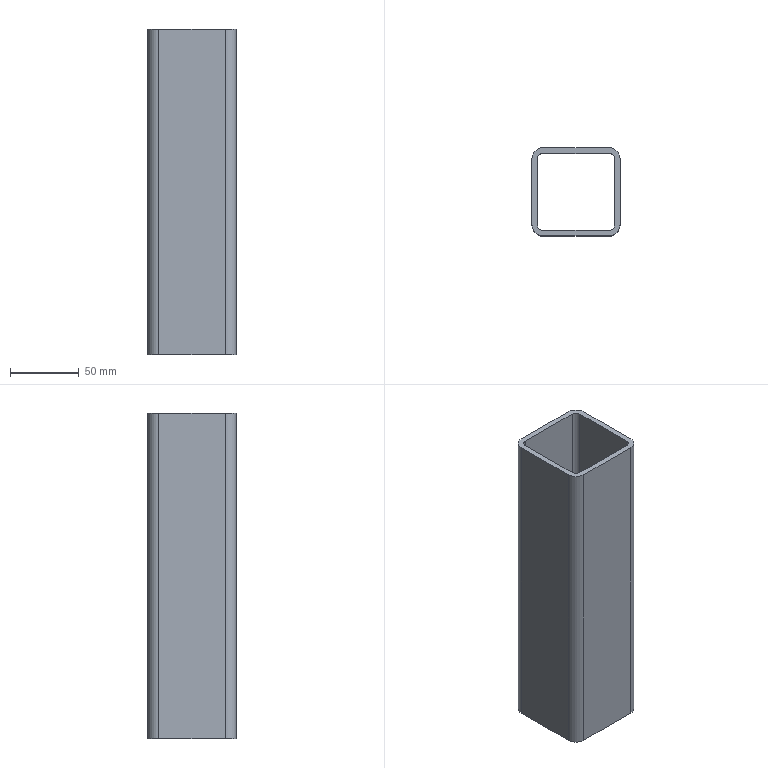Part | SolidWorks | features Extrusion 1 | 1 solid | 18 faces | box 64 x 64 x 236 mm | volume 216836 mm3 | plane 10 | cylinder 8 | commonest cylinder face diameters 8 x4 16 x4
STEP:
#1=CARTESIAN_POINT('',(-24.,32.,118.));
#2=VERTEX_POINT('',#1);
#3=CARTESIAN_POINT('',(-32.,24.,118.));
#4=VERTEX_POINT('',#3);
#5=CARTESIAN_POINT('',(-24.,24.,118.));
#6=DIRECTION('',(0.,0.,1.));
#7=DIRECTION('',(1.,0.,0.));
#8=AXIS2_PLACEMENT_3D('',#5,#6,#7);
#9=CIRCLE('',#8,8.);
#10=EDGE_CURVE('',#2,#4,#9,.T.);
#11=ORIENTED_EDGE('',*,*,#10,.T.);
#12=CARTESIAN_POINT('',(-32.,-24.,118.));
#13=VERTEX_POINT('',#12);
#14=CARTESIAN_POINT('',(-32.,24.,118.));
#15=DIRECTION('',(0.,-1.,0.));
#16=VECTOR('',#15,1000.);
#17=LINE('',#14,#16);
#18=EDGE_CURVE('',#4,#13,#17,.T.);
#19=ORIENTED_EDGE('',*,*,#18,.T.);
#20=CARTESIAN_POINT('',(-24.,-32.,118.));
#21=VERTEX_POINT('',#20);
#22=CARTESIAN_POINT('',(-24.,-24.,118.));
#23=DIRECTION('',(0.,0.,1.));
#24=DIRECTION('',(-1.,0.,0.));
#25=AXIS2_PLACEMENT_3D('',#22,#23,#24);
#26=CIRCLE('',#25,8.);
#27=EDGE_CURVE('',#13,#21,#26,.T.);
#28=ORIENTED_EDGE('',*,*,#27,.T.);
#29=CARTESIAN_POINT('',(24.,-32.,118.));
#30=VERTEX_POINT('',#29);
#31=CARTESIAN_POINT('',(24.,-32.,118.));
#32=DIRECTION('',(1.,0.,0.));
#33=VECTOR('',#32,1000.);
#34=LINE('',#31,#33);
#35=EDGE_CURVE('',#21,#30,#34,.T.);
#36=ORIENTED_EDGE('',*,*,#35,.T.);
#37=CARTESIAN_POINT('',(32.,-24.,118.));
#38=VERTEX_POINT('',#37);
#39=CARTESIAN_POINT('',(24.,-24.,118.));
#40=DIRECTION('',(0.,0.,1.));
#41=DIRECTION('',(1.,0.,0.));
#42=AXIS2_PLACEMENT_3D('',#39,#40,#41);
#43=CIRCLE('',#42,8.);
#44=EDGE_CURVE('',#30,#38,#43,.T.);
#45=ORIENTED_EDGE('',*,*,#44,.T.);
#46=CARTESIAN_POINT('',(32.,24.,118.));
#47=VERTEX_POINT('',#46);
#48=CARTESIAN_POINT('',(32.,-24.,118.));
#49=DIRECTION('',(0.,1.,0.));
#50=VECTOR('',#49,1000.);
#51=LINE('',#48,#50);
#52=EDGE_CURVE('',#38,#47,#51,.T.);
#53=ORIENTED_EDGE('',*,*,#52,.T.);
#54=CARTESIAN_POINT('',(24.,32.,118.));
#55=VERTEX_POINT('',#54);
#56=CARTESIAN_POINT('',(24.,24.,118.));
#57=DIRECTION('',(0.,0.,1.));
#58=DIRECTION('',(-1.,0.,0.));
#59=AXIS2_PLACEMENT_3D('',#56,#57,#58);
#60=CIRCLE('',#59,8.);
#61=EDGE_CURVE('',#47,#55,#60,.T.);
#62=ORIENTED_EDGE('',*,*,#61,.T.);
#63=CARTESIAN_POINT('',(0.,32.,118.));
#64=DIRECTION('',(-1.,0.,0.));
#65=VECTOR('',#64,1000.);
#66=LINE('',#63,#65);
#67=EDGE_CURVE('',#55,#2,#66,.T.);
#68=ORIENTED_EDGE('',*,*,#67,.T.);
#69=EDGE_LOOP('',(#11,#19,#28,#36,#45,#53,#62,#68));
#70=FACE_OUTER_BOUND('',#69,.T.);
#71=CARTESIAN_POINT('',(-28.,24.,118.));
#72=VERTEX_POINT('',#71);
#73=CARTESIAN_POINT('',(-28.,-24.,118.));
#74=VERTEX_POINT('',#73);
#75=CARTESIAN_POINT('',(-28.,24.,118.));
#76=DIRECTION('',(0.,-1.,0.));
#77=VECTOR('',#76,1000.);
#78=LINE('',#75,#77);
#79=EDGE_CURVE('',#72,#74,#78,.T.);
#80=ORIENTED_EDGE('',*,*,#79,.F.);
#81=CARTESIAN_POINT('',(-24.,28.,118.));
#82=VERTEX_POINT('',#81);
#83=CARTESIAN_POINT('',(-24.,24.,118.));
#84=DIRECTION('',(0.,0.,1.));
#85=DIRECTION('',(1.,0.,0.));
#86=AXIS2_PLACEMENT_3D('',#83,#84,#85);
#87=CIRCLE('',#86,4.);
#88=EDGE_CURVE('',#82,#72,#87,.T.);
#89=ORIENTED_EDGE('',*,*,#88,.F.);
#90=CARTESIAN_POINT('',(24.,28.,118.));
#91=VERTEX_POINT('',#90);
#92=CARTESIAN_POINT('',(0.,28.,118.));
#93=DIRECTION('',(-1.,0.,0.));
#94=VECTOR('',#93,1000.);
#95=LINE('',#92,#94);
#96=EDGE_CURVE('',#91,#82,#95,.T.);
#97=ORIENTED_EDGE('',*,*,#96,.F.);
#98=CARTESIAN_POINT('',(28.,24.,118.));
#99=VERTEX_POINT('',#98);
#100=CARTESIAN_POINT('',(24.,24.,118.));
#101=DIRECTION('',(0.,0.,1.));
#102=DIRECTION('',(-1.,0.,0.));
#103=AXIS2_PLACEMENT_3D('',#100,#101,#102);
#104=CIRCLE('',#103,4.);
#105=EDGE_CURVE('',#99,#91,#104,.T.);
#106=ORIENTED_EDGE('',*,*,#105,.F.);
#107=CARTESIAN_POINT('',(28.,-24.,118.));
#108=VERTEX_POINT('',#107);
#109=CARTESIAN_POINT('',(28.,-24.,118.));
#110=DIRECTION('',(0.,1.,0.));
#111=VECTOR('',#110,1000.);
#112=LINE('',#109,#111);
#113=EDGE_CURVE('',#108,#99,#112,.T.);
#114=ORIENTED_EDGE('',*,*,#113,.F.);
#115=CARTESIAN_POINT('',(24.,-28.,118.));
#116=VERTEX_POINT('',#115);
#117=CARTESIAN_POINT('',(24.,-24.,118.));
#118=DIRECTION('',(0.,0.,1.));
#119=DIRECTION('',(1.,0.,0.));
#120=AXIS2_PLACEMENT_3D('',#117,#118,#119);
#121=CIRCLE('',#120,4.);
#122=EDGE_CURVE('',#116,#108,#121,.T.);
#123=ORIENTED_EDGE('',*,*,#122,.F.);
#124=CARTESIAN_POINT('',(-24.,-28.,118.));
#125=VERTEX_POINT('',#124);
#126=CARTESIAN_POINT('',(24.,-28.,118.));
#127=DIRECTION('',(1.,0.,0.));
#128=VECTOR('',#127,1000.);
#129=LINE('',#126,#128);
#130=EDGE_CURVE('',#125,#116,#129,.T.);
#131=ORIENTED_EDGE('',*,*,#130,.F.);
#132=CARTESIAN_POINT('',(-24.,-24.,118.));
#133=DIRECTION('',(0.,0.,1.));
#134=DIRECTION('',(-1.,0.,0.));
#135=AXIS2_PLACEMENT_3D('',#132,#133,#134);
#136=CIRCLE('',#135,4.);
#137=EDGE_CURVE('',#74,#125,#136,.T.);
#138=ORIENTED_EDGE('',*,*,#137,.F.);
#139=EDGE_LOOP('',(#80,#89,#97,#106,#114,#123,#131,#138));
#140=FACE_BOUND('',#139,.T.);
#141=CARTESIAN_POINT('',(-24.,24.,118.));
#142=DIRECTION('',(0.,0.,1.));
#143=DIRECTION('',(1.,0.,0.));
#144=AXIS2_PLACEMENT_3D('',#141,#142,#143);
#145=PLANE('',#144);
#146=ADVANCED_FACE('',(#70,#140),#145,.T.);
#147=CARTESIAN_POINT('',(-24.,32.,-118.));
#148=VERTEX_POINT('',#147);
#149=CARTESIAN_POINT('',(-32.,24.,-118.));
#150=VERTEX_POINT('',#149);
#151=CARTESIAN_POINT('',(-24.,24.,-118.));
#152=DIRECTION('',(0.,0.,1.));
#153=DIRECTION('',(1.,0.,0.));
#154=AXIS2_PLACEMENT_3D('',#151,#152,#153);
#155=CIRCLE('',#154,8.);
#156=EDGE_CURVE('',#148,#150,#155,.T.);
#157=ORIENTED_EDGE('',*,*,#156,.F.);
#158=CARTESIAN_POINT('',(24.,32.,-118.));
#159=VERTEX_POINT('',#158);
#160=CARTESIAN_POINT('',(0.,32.,-118.));
#161=DIRECTION('',(-1.,0.,0.));
#162=VECTOR('',#161,1000.);
#163=LINE('',#160,#162);
#164=EDGE_CURVE('',#159,#148,#163,.T.);
#165=ORIENTED_EDGE('',*,*,#164,.F.);
#166=CARTESIAN_POINT('',(32.,24.,-118.));
#167=VERTEX_POINT('',#166);
#168=CARTESIAN_POINT('',(24.,24.,-118.));
#169=DIRECTION('',(0.,0.,1.));
#170=DIRECTION('',(-1.,0.,0.));
#171=AXIS2_PLACEMENT_3D('',#168,#169,#170);
#172=CIRCLE('',#171,8.);
#173=EDGE_CURVE('',#167,#159,#172,.T.);
#174=ORIENTED_EDGE('',*,*,#173,.F.);
#175=CARTESIAN_POINT('',(32.,-24.,-118.));
#176=VERTEX_POINT('',#175);
#177=CARTESIAN_POINT('',(32.,24.,-118.));
#178=DIRECTION('',(0.,1.,0.));
#179=VECTOR('',#178,1000.);
#180=LINE('',#177,#179);
#181=EDGE_CURVE('',#176,#167,#180,.T.);
#182=ORIENTED_EDGE('',*,*,#181,.F.);
#183=CARTESIAN_POINT('',(24.,-32.,-118.));
#184=VERTEX_POINT('',#183);
#185=CARTESIAN_POINT('',(24.,-24.,-118.));
#186=DIRECTION('',(0.,0.,1.));
#187=DIRECTION('',(1.,0.,0.));
#188=AXIS2_PLACEMENT_3D('',#185,#186,#187);
#189=CIRCLE('',#188,8.);
#190=EDGE_CURVE('',#184,#176,#189,.T.);
#191=ORIENTED_EDGE('',*,*,#190,.F.);
#192=CARTESIAN_POINT('',(-24.,-32.,-118.));
#193=VERTEX_POINT('',#192);
#194=CARTESIAN_POINT('',(24.,-32.,-118.));
#195=DIRECTION('',(1.,0.,0.));
#196=VECTOR('',#195,1000.);
#197=LINE('',#194,#196);
#198=EDGE_CURVE('',#193,#184,#197,.T.);
#199=ORIENTED_EDGE('',*,*,#198,.F.);
#200=CARTESIAN_POINT('',(-32.,-24.,-118.));
#201=VERTEX_POINT('',#200);
#202=CARTESIAN_POINT('',(-24.,-24.,-118.));
#203=DIRECTION('',(0.,0.,1.));
#204=DIRECTION('',(-1.,0.,0.));
#205=AXIS2_PLACEMENT_3D('',#202,#203,#204);
#206=CIRCLE('',#205,8.);
#207=EDGE_CURVE('',#201,#193,#206,.T.);
#208=ORIENTED_EDGE('',*,*,#207,.F.);
#209=CARTESIAN_POINT('',(-32.,-24.,-118.));
#210=DIRECTION('',(0.,-1.,0.));
#211=VECTOR('',#210,1000.);
#212=LINE('',#209,#211);
#213=EDGE_CURVE('',#150,#201,#212,.T.);
#214=ORIENTED_EDGE('',*,*,#213,.F.);
#215=EDGE_LOOP('',(#157,#165,#174,#182,#191,#199,#208,#214));
#216=FACE_OUTER_BOUND('',#215,.T.);
#217=CARTESIAN_POINT('',(-24.,28.,-118.));
#218=VERTEX_POINT('',#217);
#219=CARTESIAN_POINT('',(-28.,24.,-118.));
#220=VERTEX_POINT('',#219);
#221=CARTESIAN_POINT('',(-24.,24.,-118.));
#222=DIRECTION('',(0.,0.,1.));
#223=DIRECTION('',(1.,0.,0.));
#224=AXIS2_PLACEMENT_3D('',#221,#222,#223);
#225=CIRCLE('',#224,4.);
#226=EDGE_CURVE('',#218,#220,#225,.T.);
#227=ORIENTED_EDGE('',*,*,#226,.T.);
#228=CARTESIAN_POINT('',(-28.,-24.,-118.));
#229=VERTEX_POINT('',#228);
#230=CARTESIAN_POINT('',(-28.,-24.,-118.));
#231=DIRECTION('',(0.,-1.,0.));
#232=VECTOR('',#231,1000.);
#233=LINE('',#230,#232);
#234=EDGE_CURVE('',#220,#229,#233,.T.);
#235=ORIENTED_EDGE('',*,*,#234,.T.);
#236=CARTESIAN_POINT('',(-24.,-28.,-118.));
#237=VERTEX_POINT('',#236);
#238=CARTESIAN_POINT('',(-24.,-24.,-118.));
#239=DIRECTION('',(0.,0.,1.));
#240=DIRECTION('',(-1.,0.,0.));
#241=AXIS2_PLACEMENT_3D('',#238,#239,#240);
#242=CIRCLE('',#241,4.);
#243=EDGE_CURVE('',#229,#237,#242,.T.);
#244=ORIENTED_EDGE('',*,*,#243,.T.);
#245=CARTESIAN_POINT('',(24.,-28.,-118.));
#246=VERTEX_POINT('',#245);
#247=CARTESIAN_POINT('',(24.,-28.,-118.));
#248=DIRECTION('',(1.,0.,0.));
#249=VECTOR('',#248,1000.);
#250=LINE('',#247,#249);
#251=EDGE_CURVE('',#237,#246,#250,.T.);
#252=ORIENTED_EDGE('',*,*,#251,.T.);
#253=CARTESIAN_POINT('',(28.,-24.,-118.));
#254=VERTEX_POINT('',#253);
#255=CARTESIAN_POINT('',(24.,-24.,-118.));
#256=DIRECTION('',(0.,0.,1.));
#257=DIRECTION('',(1.,0.,0.));
#258=AXIS2_PLACEMENT_3D('',#255,#256,#257);
#259=CIRCLE('',#258,4.);
#260=EDGE_CURVE('',#246,#254,#259,.T.);
#261=ORIENTED_EDGE('',*,*,#260,.T.);
#262=CARTESIAN_POINT('',(28.,24.,-118.));
#263=VERTEX_POINT('',#262);
#264=CARTESIAN_POINT('',(28.,24.,-118.));
#265=DIRECTION('',(0.,1.,0.));
#266=VECTOR('',#265,1000.);
#267=LINE('',#264,#266);
#268=EDGE_CURVE('',#254,#263,#267,.T.);
#269=ORIENTED_EDGE('',*,*,#268,.T.);
#270=CARTESIAN_POINT('',(24.,28.,-118.));
#271=VERTEX_POINT('',#270);
#272=CARTESIAN_POINT('',(24.,24.,-118.));
#273=DIRECTION('',(0.,0.,1.));
#274=DIRECTION('',(-1.,0.,0.));
#275=AXIS2_PLACEMENT_3D('',#272,#273,#274);
#276=CIRCLE('',#275,4.);
#277=EDGE_CURVE('',#263,#271,#276,.T.);
#278=ORIENTED_EDGE('',*,*,#277,.T.);
#279=CARTESIAN_POINT('',(0.,28.,-118.));
#280=DIRECTION('',(-1.,0.,0.));
#281=VECTOR('',#280,1000.);
#282=LINE('',#279,#281);
#283=EDGE_CURVE('',#271,#218,#282,.T.);
#284=ORIENTED_EDGE('',*,*,#283,.T.);
#285=EDGE_LOOP('',(#227,#235,#244,#252,#261,#269,#278,#284));
#286=FACE_BOUND('',#285,.T.);
#287=CARTESIAN_POINT('',(-24.,24.,-118.));
#288=DIRECTION('',(0.,0.,1.));
#289=DIRECTION('',(1.,0.,0.));
#290=AXIS2_PLACEMENT_3D('',#287,#288,#289);
#291=PLANE('',#290);
#292=ADVANCED_FACE('',(#216,#286),#291,.F.);
#293=ORIENTED_EDGE('',*,*,#156,.T.);
#294=CARTESIAN_POINT('',(-32.,24.,118.));
#295=DIRECTION('',(0.,0.,-1.));
#296=VECTOR('',#295,1000.);
#297=LINE('',#294,#296);
#298=EDGE_CURVE('',#4,#150,#297,.T.);
#299=ORIENTED_EDGE('',*,*,#298,.F.);
#300=ORIENTED_EDGE('',*,*,#10,.F.);
#301=CARTESIAN_POINT('',(-24.,32.,118.));
#302=DIRECTION('',(0.,0.,-1.));
#303=VECTOR('',#302,1000.);
#304=LINE('',#301,#303);
#305=EDGE_CURVE('',#2,#148,#304,.T.);
#306=ORIENTED_EDGE('',*,*,#305,.T.);
#307=EDGE_LOOP('',(#293,#299,#300,#306));
#308=FACE_OUTER_BOUND('',#307,.T.);
#309=CARTESIAN_POINT('',(-24.,24.,118.));
#310=DIRECTION('',(0.,0.,-1.));
#311=DIRECTION('',(-1.,0.,0.));
#312=AXIS2_PLACEMENT_3D('',#309,#310,#311);
#313=CYLINDRICAL_SURFACE('',#312,8.);
#314=ADVANCED_FACE('',(#308),#313,.T.);
#315=ORIENTED_EDGE('',*,*,#213,.T.);
#316=CARTESIAN_POINT('',(-32.,-24.,118.));
#317=DIRECTION('',(0.,0.,-1.));
#318=VECTOR('',#317,1000.);
#319=LINE('',#316,#318);
#320=EDGE_CURVE('',#13,#201,#319,.T.);
#321=ORIENTED_EDGE('',*,*,#320,.F.);
#322=ORIENTED_EDGE('',*,*,#18,.F.);
#323=ORIENTED_EDGE('',*,*,#298,.T.);
#324=EDGE_LOOP('',(#315,#321,#322,#323));
#325=FACE_OUTER_BOUND('',#324,.T.);
#326=CARTESIAN_POINT('',(-32.,-24.,118.));
#327=DIRECTION('',(1.,0.,0.));
#328=DIRECTION('',(0.,0.,-1.));
#329=AXIS2_PLACEMENT_3D('',#326,#327,#328);
#330=PLANE('',#329);
#331=ADVANCED_FACE('',(#325),#330,.F.);
#332=ORIENTED_EDGE('',*,*,#207,.T.);
#333=CARTESIAN_POINT('',(-24.,-32.,118.));
#334=DIRECTION('',(0.,0.,-1.));
#335=VECTOR('',#334,1000.);
#336=LINE('',#333,#335);
#337=EDGE_CURVE('',#21,#193,#336,.T.);
#338=ORIENTED_EDGE('',*,*,#337,.F.);
#339=ORIENTED_EDGE('',*,*,#27,.F.);
#340=ORIENTED_EDGE('',*,*,#320,.T.);
#341=EDGE_LOOP('',(#332,#338,#339,#340));
#342=FACE_OUTER_BOUND('',#341,.T.);
#343=CARTESIAN_POINT('',(-24.,-24.,118.));
#344=DIRECTION('',(0.,0.,-1.));
#345=DIRECTION('',(-1.,0.,0.));
#346=AXIS2_PLACEMENT_3D('',#343,#344,#345);
#347=CYLINDRICAL_SURFACE('',#346,8.);
#348=ADVANCED_FACE('',(#342),#347,.T.);
#349=ORIENTED_EDGE('',*,*,#198,.T.);
#350=CARTESIAN_POINT('',(24.,-32.,118.));
#351=DIRECTION('',(0.,0.,-1.));
#352=VECTOR('',#351,1000.);
#353=LINE('',#350,#352);
#354=EDGE_CURVE('',#30,#184,#353,.T.);
#355=ORIENTED_EDGE('',*,*,#354,.F.);
#356=ORIENTED_EDGE('',*,*,#35,.F.);
#357=ORIENTED_EDGE('',*,*,#337,.T.);
#358=EDGE_LOOP('',(#349,#355,#356,#357));
#359=FACE_OUTER_BOUND('',#358,.T.);
#360=CARTESIAN_POINT('',(24.,-32.,118.));
#361=DIRECTION('',(0.,1.,0.));
#362=DIRECTION('',(-1.,0.,0.));
#363=AXIS2_PLACEMENT_3D('',#360,#361,#362);
#364=PLANE('',#363);
#365=ADVANCED_FACE('',(#359),#364,.F.);
#366=ORIENTED_EDGE('',*,*,#190,.T.);
#367=CARTESIAN_POINT('',(32.,-24.,118.));
#368=DIRECTION('',(0.,0.,-1.));
#369=VECTOR('',#368,1000.);
#370=LINE('',#367,#369);
#371=EDGE_CURVE('',#38,#176,#370,.T.);
#372=ORIENTED_EDGE('',*,*,#371,.F.);
#373=ORIENTED_EDGE('',*,*,#44,.F.);
#374=ORIENTED_EDGE('',*,*,#354,.T.);
#375=EDGE_LOOP('',(#366,#372,#373,#374));
#376=FACE_OUTER_BOUND('',#375,.T.);
#377=CARTESIAN_POINT('',(24.,-24.,118.));
#378=DIRECTION('',(0.,0.,-1.));
#379=DIRECTION('',(-1.,0.,0.));
#380=AXIS2_PLACEMENT_3D('',#377,#378,#379);
#381=CYLINDRICAL_SURFACE('',#380,8.);
#382=ADVANCED_FACE('',(#376),#381,.T.);
#383=ORIENTED_EDGE('',*,*,#181,.T.);
#384=CARTESIAN_POINT('',(32.,24.,118.));
#385=DIRECTION('',(0.,0.,-1.));
#386=VECTOR('',#385,1000.);
#387=LINE('',#384,#386);
#388=EDGE_CURVE('',#47,#167,#387,.T.);
#389=ORIENTED_EDGE('',*,*,#388,.F.);
#390=ORIENTED_EDGE('',*,*,#52,.F.);
#391=ORIENTED_EDGE('',*,*,#371,.T.);
#392=EDGE_LOOP('',(#383,#389,#390,#391));
#393=FACE_OUTER_BOUND('',#392,.T.);
#394=CARTESIAN_POINT('',(32.,24.,118.));
#395=DIRECTION('',(-1.,0.,0.));
#396=DIRECTION('',(0.,0.,1.));
#397=AXIS2_PLACEMENT_3D('',#394,#395,#396);
#398=PLANE('',#397);
#399=ADVANCED_FACE('',(#393),#398,.F.);
#400=ORIENTED_EDGE('',*,*,#173,.T.);
#401=CARTESIAN_POINT('',(24.,32.,118.));
#402=DIRECTION('',(0.,0.,-1.));
#403=VECTOR('',#402,1000.);
#404=LINE('',#401,#403);
#405=EDGE_CURVE('',#55,#159,#404,.T.);
#406=ORIENTED_EDGE('',*,*,#405,.F.);
#407=ORIENTED_EDGE('',*,*,#61,.F.);
#408=ORIENTED_EDGE('',*,*,#388,.T.);
#409=EDGE_LOOP('',(#400,#406,#407,#408));
#410=FACE_OUTER_BOUND('',#409,.T.);
#411=CARTESIAN_POINT('',(24.,24.,118.));
#412=DIRECTION('',(0.,0.,-1.));
#413=DIRECTION('',(-1.,0.,0.));
#414=AXIS2_PLACEMENT_3D('',#411,#412,#413);
#415=CYLINDRICAL_SURFACE('',#414,8.);
#416=ADVANCED_FACE('',(#410),#415,.T.);
#417=ORIENTED_EDGE('',*,*,#164,.T.);
#418=ORIENTED_EDGE('',*,*,#305,.F.);
#419=ORIENTED_EDGE('',*,*,#67,.F.);
#420=ORIENTED_EDGE('',*,*,#405,.T.);
#421=EDGE_LOOP('',(#417,#418,#419,#420));
#422=FACE_OUTER_BOUND('',#421,.T.);
#423=CARTESIAN_POINT('',(0.,32.,118.));
#424=DIRECTION('',(0.,-1.,0.));
#425=DIRECTION('',(0.,0.,-1.));
#426=AXIS2_PLACEMENT_3D('',#423,#424,#425);
#427=PLANE('',#426);
#428=ADVANCED_FACE('',(#422),#427,.F.);
#429=ORIENTED_EDGE('',*,*,#226,.F.);
#430=CARTESIAN_POINT('',(-24.,28.,118.));
#431=DIRECTION('',(0.,0.,-1.));
#432=VECTOR('',#431,1000.);
#433=LINE('',#430,#432);
#434=EDGE_CURVE('',#82,#218,#433,.T.);
#435=ORIENTED_EDGE('',*,*,#434,.F.);
#436=ORIENTED_EDGE('',*,*,#88,.T.);
#437=CARTESIAN_POINT('',(-28.,24.,118.));
#438=DIRECTION('',(0.,0.,-1.));
#439=VECTOR('',#438,1000.);
#440=LINE('',#437,#439);
#441=EDGE_CURVE('',#72,#220,#440,.T.);
#442=ORIENTED_EDGE('',*,*,#441,.T.);
#443=EDGE_LOOP('',(#429,#435,#436,#442));
#444=FACE_OUTER_BOUND('',#443,.T.);
#445=CARTESIAN_POINT('',(-24.,24.,118.));
#446=DIRECTION('',(0.,0.,-1.));
#447=DIRECTION('',(-1.,0.,0.));
#448=AXIS2_PLACEMENT_3D('',#445,#446,#447);
#449=CYLINDRICAL_SURFACE('',#448,4.);
#450=ADVANCED_FACE('',(#444),#449,.F.);
#451=ORIENTED_EDGE('',*,*,#234,.F.);
#452=ORIENTED_EDGE('',*,*,#441,.F.);
#453=ORIENTED_EDGE('',*,*,#79,.T.);
#454=CARTESIAN_POINT('',(-28.,-24.,118.));
#455=DIRECTION('',(0.,0.,-1.));
#456=VECTOR('',#455,1000.);
#457=LINE('',#454,#456);
#458=EDGE_CURVE('',#74,#229,#457,.T.);
#459=ORIENTED_EDGE('',*,*,#458,.T.);
#460=EDGE_LOOP('',(#451,#452,#453,#459));
#461=FACE_OUTER_BOUND('',#460,.T.);
#462=CARTESIAN_POINT('',(-28.,-24.,118.));
#463=DIRECTION('',(1.,0.,0.));
#464=DIRECTION('',(0.,1.,0.));
#465=AXIS2_PLACEMENT_3D('',#462,#463,#464);
#466=PLANE('',#465);
#467=ADVANCED_FACE('',(#461),#466,.T.);
#468=ORIENTED_EDGE('',*,*,#243,.F.);
#469=ORIENTED_EDGE('',*,*,#458,.F.);
#470=ORIENTED_EDGE('',*,*,#137,.T.);
#471=CARTESIAN_POINT('',(-24.,-28.,118.));
#472=DIRECTION('',(0.,0.,-1.));
#473=VECTOR('',#472,1000.);
#474=LINE('',#471,#473);
#475=EDGE_CURVE('',#125,#237,#474,.T.);
#476=ORIENTED_EDGE('',*,*,#475,.T.);
#477=EDGE_LOOP('',(#468,#469,#470,#476));
#478=FACE_OUTER_BOUND('',#477,.T.);
#479=CARTESIAN_POINT('',(-24.,-24.,118.));
#480=DIRECTION('',(0.,0.,-1.));
#481=DIRECTION('',(-1.,0.,0.));
#482=AXIS2_PLACEMENT_3D('',#479,#480,#481);
#483=CYLINDRICAL_SURFACE('',#482,4.);
#484=ADVANCED_FACE('',(#478),#483,.F.);
#485=ORIENTED_EDGE('',*,*,#251,.F.);
#486=ORIENTED_EDGE('',*,*,#475,.F.);
#487=ORIENTED_EDGE('',*,*,#130,.T.);
#488=CARTESIAN_POINT('',(24.,-28.,118.));
#489=DIRECTION('',(0.,0.,-1.));
#490=VECTOR('',#489,1000.);
#491=LINE('',#488,#490);
#492=EDGE_CURVE('',#116,#246,#491,.T.);
#493=ORIENTED_EDGE('',*,*,#492,.T.);
#494=EDGE_LOOP('',(#485,#486,#487,#493));
#495=FACE_OUTER_BOUND('',#494,.T.);
#496=CARTESIAN_POINT('',(24.,-28.,118.));
#497=DIRECTION('',(0.,1.,0.));
#498=DIRECTION('',(-1.,0.,0.));
#499=AXIS2_PLACEMENT_3D('',#496,#497,#498);
#500=PLANE('',#499);
#501=ADVANCED_FACE('',(#495),#500,.T.);
#502=ORIENTED_EDGE('',*,*,#260,.F.);
#503=ORIENTED_EDGE('',*,*,#492,.F.);
#504=ORIENTED_EDGE('',*,*,#122,.T.);
#505=CARTESIAN_POINT('',(28.,-24.,118.));
#506=DIRECTION('',(0.,0.,-1.));
#507=VECTOR('',#506,1000.);
#508=LINE('',#505,#507);
#509=EDGE_CURVE('',#108,#254,#508,.T.);
#510=ORIENTED_EDGE('',*,*,#509,.T.);
#511=EDGE_LOOP('',(#502,#503,#504,#510));
#512=FACE_OUTER_BOUND('',#511,.T.);
#513=CARTESIAN_POINT('',(24.,-24.,118.));
#514=DIRECTION('',(0.,0.,-1.));
#515=DIRECTION('',(-1.,0.,0.));
#516=AXIS2_PLACEMENT_3D('',#513,#514,#515);
#517=CYLINDRICAL_SURFACE('',#516,4.);
#518=ADVANCED_FACE('',(#512),#517,.F.);
#519=ORIENTED_EDGE('',*,*,#268,.F.);
#520=ORIENTED_EDGE('',*,*,#509,.F.);
#521=ORIENTED_EDGE('',*,*,#113,.T.);
#522=CARTESIAN_POINT('',(28.,24.,118.));
#523=DIRECTION('',(0.,0.,-1.));
#524=VECTOR('',#523,1000.);
#525=LINE('',#522,#524);
#526=EDGE_CURVE('',#99,#263,#525,.T.);
#527=ORIENTED_EDGE('',*,*,#526,.T.);
#528=EDGE_LOOP('',(#519,#520,#521,#527));
#529=FACE_OUTER_BOUND('',#528,.T.);
#530=CARTESIAN_POINT('',(28.,24.,118.));
#531=DIRECTION('',(-1.,0.,0.));
#532=DIRECTION('',(0.,-1.,0.));
#533=AXIS2_PLACEMENT_3D('',#530,#531,#532);
#534=PLANE('',#533);
#535=ADVANCED_FACE('',(#529),#534,.T.);
#536=ORIENTED_EDGE('',*,*,#277,.F.);
#537=ORIENTED_EDGE('',*,*,#526,.F.);
#538=ORIENTED_EDGE('',*,*,#105,.T.);
#539=CARTESIAN_POINT('',(24.,28.,118.));
#540=DIRECTION('',(0.,0.,-1.));
#541=VECTOR('',#540,1000.);
#542=LINE('',#539,#541);
#543=EDGE_CURVE('',#91,#271,#542,.T.);
#544=ORIENTED_EDGE('',*,*,#543,.T.);
#545=EDGE_LOOP('',(#536,#537,#538,#544));
#546=FACE_OUTER_BOUND('',#545,.T.);
#547=CARTESIAN_POINT('',(24.,24.,118.));
#548=DIRECTION('',(0.,0.,-1.));
#549=DIRECTION('',(-1.,0.,0.));
#550=AXIS2_PLACEMENT_3D('',#547,#548,#549);
#551=CYLINDRICAL_SURFACE('',#550,4.);
#552=ADVANCED_FACE('',(#546),#551,.F.);
#553=ORIENTED_EDGE('',*,*,#283,.F.);
#554=ORIENTED_EDGE('',*,*,#543,.F.);
#555=ORIENTED_EDGE('',*,*,#96,.T.);
#556=ORIENTED_EDGE('',*,*,#434,.T.);
#557=EDGE_LOOP('',(#553,#554,#555,#556));
#558=FACE_OUTER_BOUND('',#557,.T.);
#559=CARTESIAN_POINT('',(0.,28.,118.));
#560=DIRECTION('',(0.,-1.,0.));
#561=DIRECTION('',(0.,0.,-1.));
#562=AXIS2_PLACEMENT_3D('',#559,#560,#561);
#563=PLANE('',#562);
#564=ADVANCED_FACE('',(#558),#563,.T.);
#565=CLOSED_SHELL('',(#146,#292,#314,#331,#348,#365,#382,#399,#416,#428,#450,#467,#484,#501,#518,#535,#552,#564));
#566=MANIFOLD_SOLID_BREP('',#565);
#567=CARTESIAN_POINT('',(0.,0.,0.));
#568=DIRECTION('',(0.,0.,1.));
#569=DIRECTION('',(1.,0.,0.));
#570=AXIS2_PLACEMENT_3D('',#567,#568,#569);
#571=(LENGTH_UNIT()NAMED_UNIT(*)SI_UNIT(.MILLI.,.METRE.));
#572=UNCERTAINTY_MEASURE_WITH_UNIT(LENGTH_MEASURE(0.00001),#571,'','');
#573=(NAMED_UNIT(*)PLANE_ANGLE_UNIT()SI_UNIT($,.RADIAN.));
#574=(NAMED_UNIT(*)SI_UNIT($,.STERADIAN.)SOLID_ANGLE_UNIT());
#575=(GEOMETRIC_REPRESENTATION_CONTEXT(3)GLOBAL_UNCERTAINTY_ASSIGNED_CONTEXT((#572))GLOBAL_UNIT_ASSIGNED_CONTEXT((#571,#573,#574))REPRESENTATION_CONTEXT('',''));
#576=ADVANCED_BREP_SHAPE_REPRESENTATION('',(#566,#570),#575);